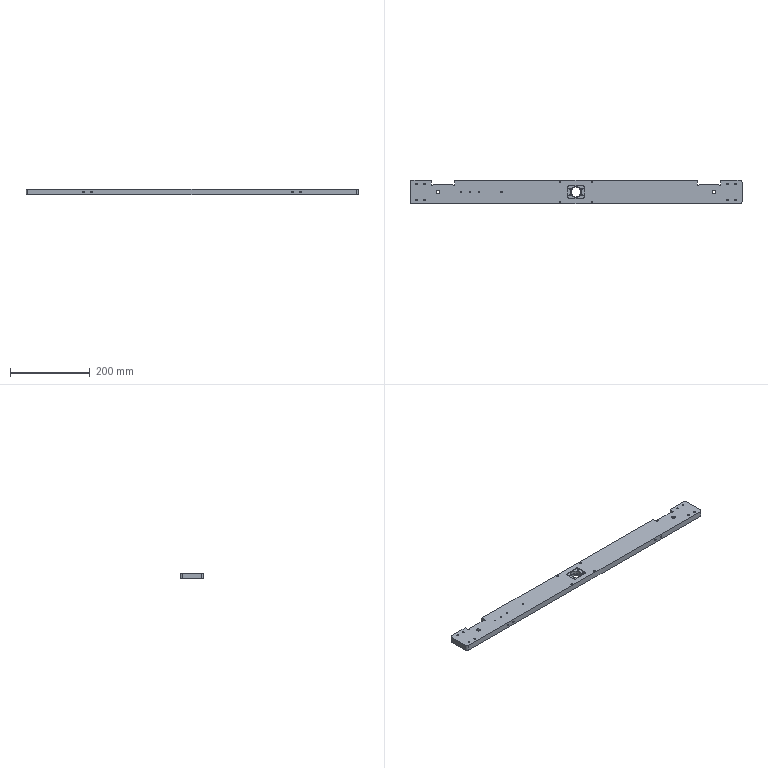Part | STEP file | front return support plate | 1 solid | 136 faces | box 835 x 60 x 15 mm | volume 710193 mm3 | cylinder 83 | cone 30 | plane 23 | commonest cylinder face diameters 4.2 x40 3.3 x16 4 x7 6 x4 9 x4 10 x4